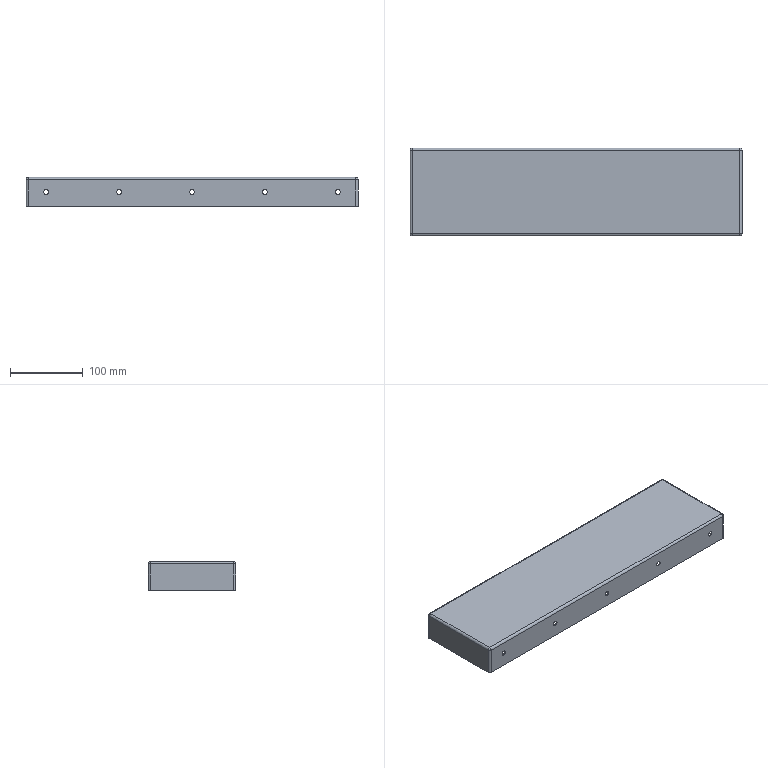Part | SolidWorks | features Extrusion 1, Fillet 1, HoleWzd 1, Shell 1 | 1 solid | 55 faces | box 455 x 120 x 40 mm | volume 145562 mm3 | cylinder 36 | plane 11 | sphere 8 | commonest cylinder face diameters 6.6 x20 3 x8 6 x8